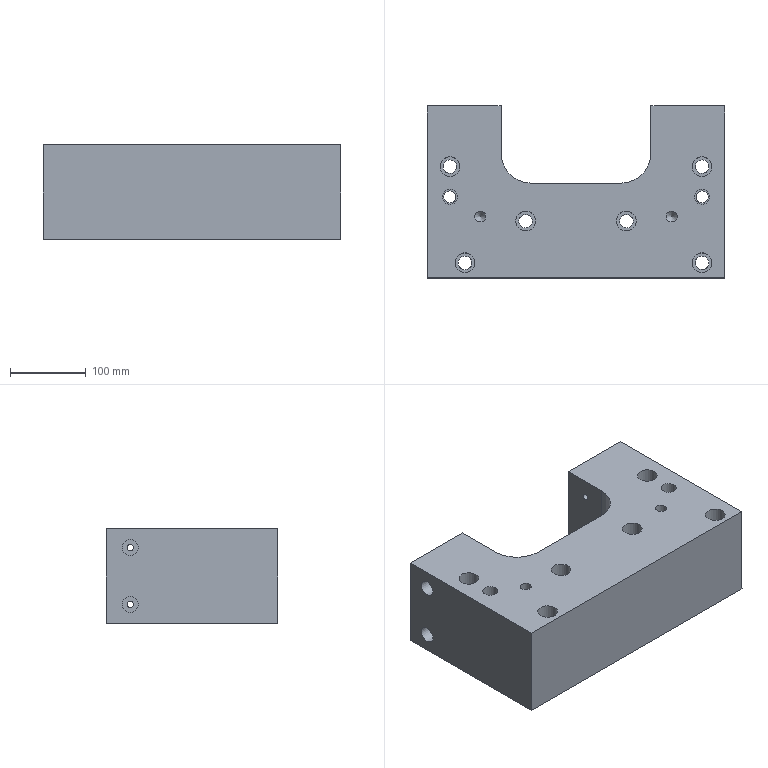Part | STEP file | lll_id546_x_t | 1 solid | 65 faces | box 393 x 227 x 125 mm | volume 8158779 mm3 | cylinder 34 | plane 25 | cone 6 | commonest cylinder face diameters 18.009 x6 26.008 x6 8.5 x4 8.506 x4 21 x4 14.506 x2